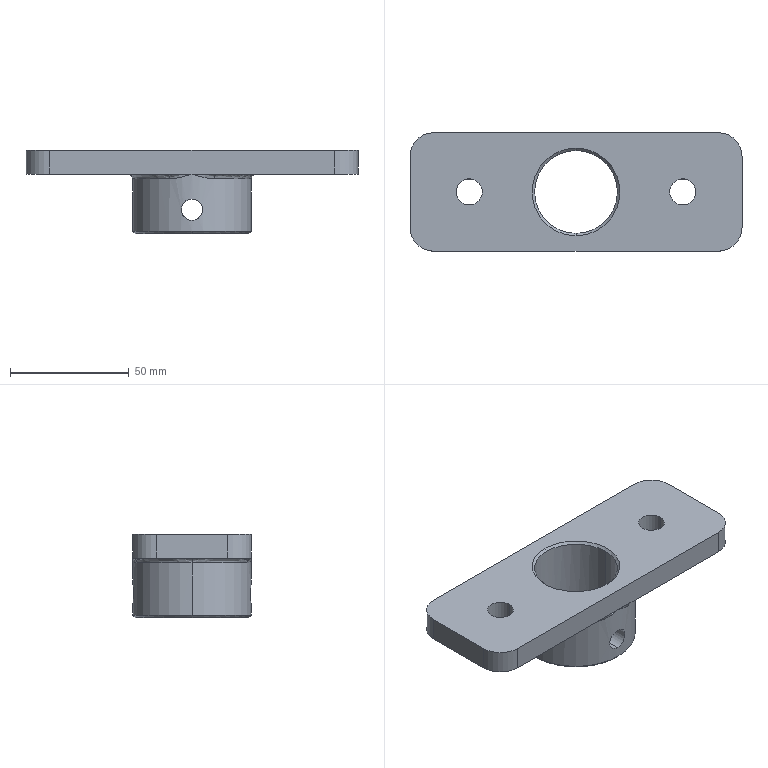Part | SolidWorks | features BaseBody 1 | 1 solid | 37 faces | box 140 x 50 x 35 mm | volume 81620 mm3 | cylinder 16 | plane 8 | spline 7 | cone 6 | commonest cylinder face diameters 9 x4 11 x4 20 x4 35 x2 50 x2